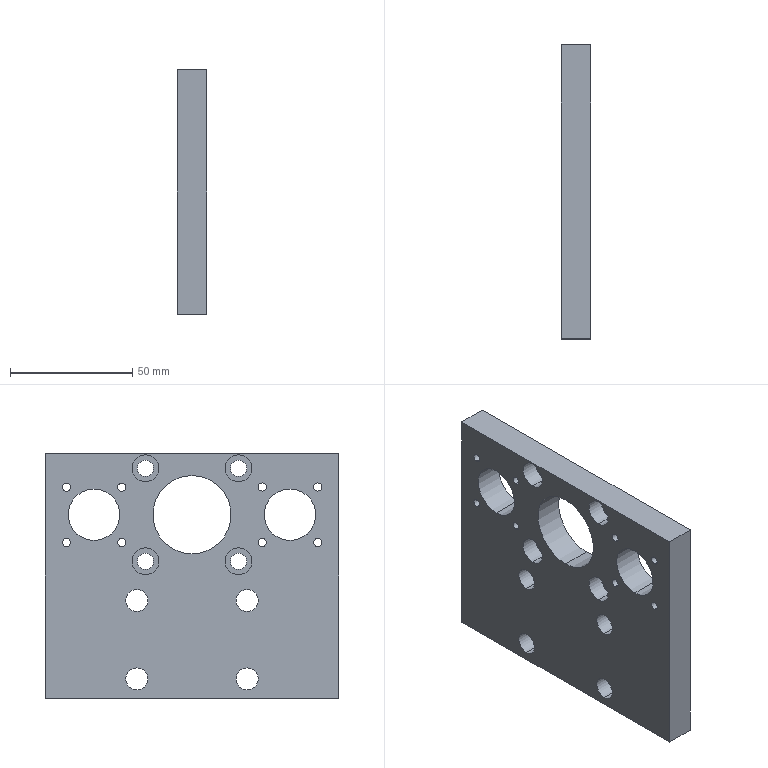Part | STEP file | X77B-01003a | 1 solid | 56 faces | box 12 x 120 x 100 mm | volume 118865 mm3 | cylinder 46 | plane 10 | commonest cylinder face diameters 3.3 x16 6.6 x8 9 x8 11 x8 21 x4 32 x2